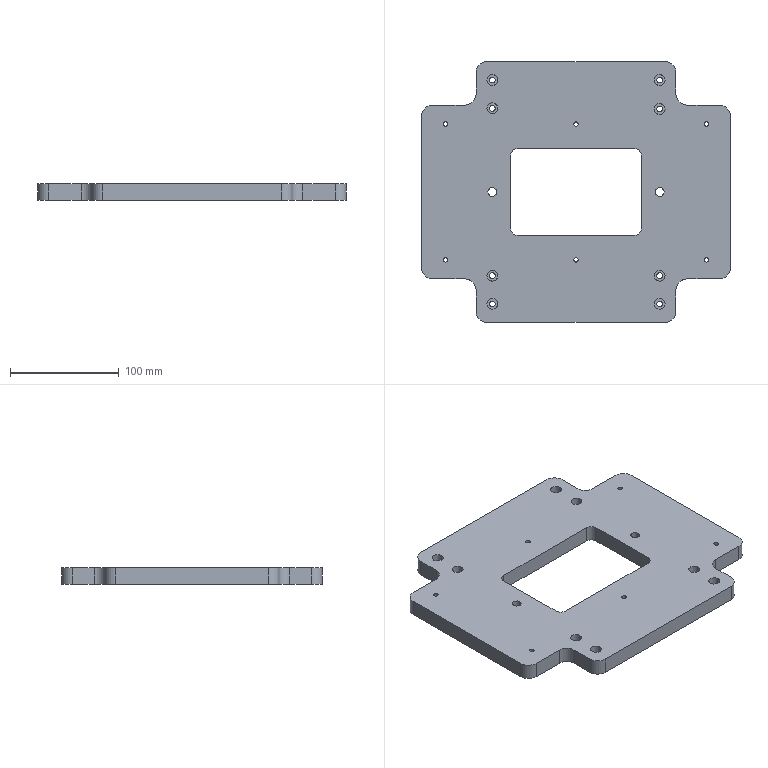Part | 1 solid | 67 faces | box 284 x 240 x 15 mm | volume 746790 mm3 | cylinder 41 | plane 26 | commonest cylinder face diameters 20 x12 5.3 x8 10 x8 4.134 x6 12 x4 8 x2